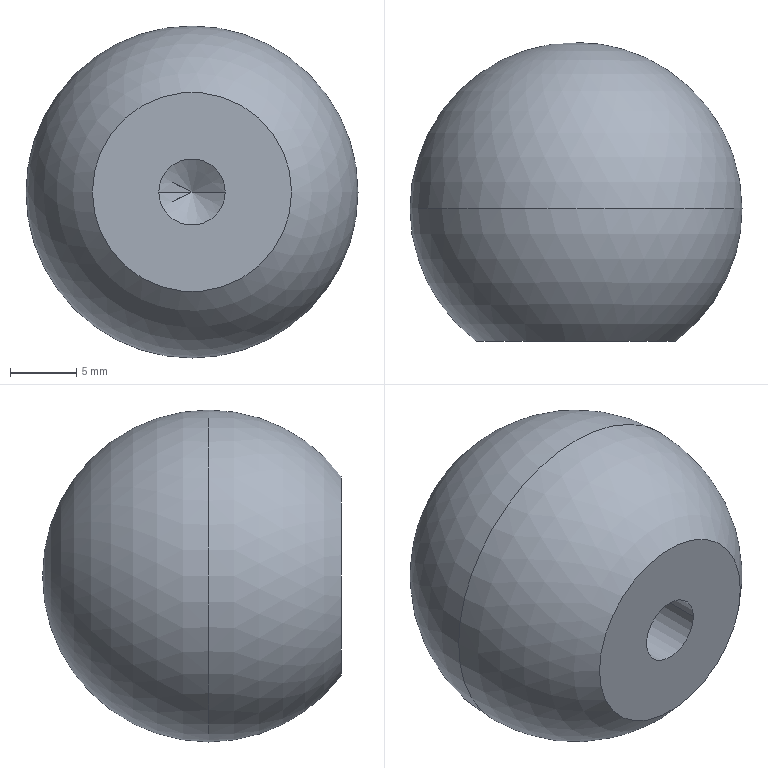Part | NX | 1 solid | 7 faces | box 25 x 22.5 x 25 mm | volume 7726 mm3 | sphere 2 | cone 2 | cylinder 2 | plane 1 | commonest cylinder face diameters 5 x2
STEP:
#1=CARTESIAN_POINT('',(-7.5,-10.,0.));
#2=VERTEX_POINT('',#1);
#3=CARTESIAN_POINT('',(7.5,-10.,0.));
#4=VERTEX_POINT('',#3);
#5=CARTESIAN_POINT('',(0.,-10.,0.));
#6=DIRECTION('',(0.,1.,0.));
#7=DIRECTION('',(-1.,0.,0.));
#8=AXIS2_PLACEMENT_3D('',#5,#6,#7);
#9=CIRCLE('',#8,7.5);
#10=EDGE_CURVE('',#2,#4,#9,.T.);
#11=ORIENTED_EDGE('',*,*,#10,.F.);
#12=CARTESIAN_POINT('',(0.,-10.,0.));
#13=DIRECTION('',(0.,1.,0.));
#14=DIRECTION('',(-1.,0.,0.));
#15=AXIS2_PLACEMENT_3D('',#12,#13,#14);
#16=CIRCLE('',#15,7.5);
#17=EDGE_CURVE('',#4,#2,#16,.T.);
#18=ORIENTED_EDGE('',*,*,#17,.F.);
#19=EDGE_LOOP('',(#11,#18));
#20=FACE_BOUND('',#19,.T.);
#21=CARTESIAN_POINT('',(-2.5,-10.,0.));
#22=VERTEX_POINT('',#21);
#23=CARTESIAN_POINT('',(2.5,-10.,0.));
#24=VERTEX_POINT('',#23);
#25=CARTESIAN_POINT('',(0.,-10.,0.));
#26=DIRECTION('',(0.,-1.,0.));
#27=DIRECTION('',(1.,0.,0.));
#28=AXIS2_PLACEMENT_3D('',#25,#26,#27);
#29=CIRCLE('',#28,2.5);
#30=EDGE_CURVE('',#22,#24,#29,.T.);
#31=ORIENTED_EDGE('',*,*,#30,.F.);
#32=CARTESIAN_POINT('',(0.,-10.,0.));
#33=DIRECTION('',(0.,-1.,0.));
#34=DIRECTION('',(1.,0.,0.));
#35=AXIS2_PLACEMENT_3D('',#32,#33,#34);
#36=CIRCLE('',#35,2.5);
#37=EDGE_CURVE('',#24,#22,#36,.T.);
#38=ORIENTED_EDGE('',*,*,#37,.F.);
#39=EDGE_LOOP('',(#31,#38));
#40=FACE_BOUND('',#39,.T.);
#41=CARTESIAN_POINT('',(0.,-10.,0.));
#42=DIRECTION('',(0.,-1.,0.));
#43=DIRECTION('',(0.,0.,-1.));
#44=AXIS2_PLACEMENT_3D('',#41,#42,#43);
#45=PLANE('',#44);
#46=ADVANCED_FACE('',(#20,#40),#45,.T.);
#47=CARTESIAN_POINT('',(12.5,0.,0.));
#48=VERTEX_POINT('',#47);
#49=CARTESIAN_POINT('',(-12.5,0.,0.));
#50=VERTEX_POINT('',#49);
#51=CARTESIAN_POINT('',(0.,0.,0.));
#52=DIRECTION('',(0.,1.,0.));
#53=DIRECTION('',(1.,0.,0.));
#54=AXIS2_PLACEMENT_3D('',#51,#52,#53);
#55=CIRCLE('',#54,12.5);
#56=EDGE_CURVE('',#48,#50,#55,.T.);
#57=ORIENTED_EDGE('',*,*,#56,.T.);
#58=CARTESIAN_POINT('',(0.,0.,0.));
#59=DIRECTION('',(0.,1.,0.));
#60=DIRECTION('',(1.,0.,0.));
#61=AXIS2_PLACEMENT_3D('',#58,#59,#60);
#62=CIRCLE('',#61,12.5);
#63=EDGE_CURVE('',#50,#48,#62,.T.);
#64=ORIENTED_EDGE('',*,*,#63,.T.);
#65=EDGE_LOOP('',(#57,#64));
#66=FACE_BOUND('',#65,.T.);
#67=CARTESIAN_POINT('',(0.,0.,0.));
#68=DIRECTION('',(0.,1.,0.));
#69=DIRECTION('',(1.,0.,0.));
#70=AXIS2_PLACEMENT_3D('',#67,#68,#69);
#71=SPHERICAL_SURFACE('',#70,12.5);
#72=ADVANCED_FACE('',(#66),#71,.T.);
#73=CARTESIAN_POINT('',(2.5,1.,0.));
#74=VERTEX_POINT('',#73);
#75=CARTESIAN_POINT('',(-2.5,1.,0.));
#76=VERTEX_POINT('',#75);
#77=CARTESIAN_POINT('',(0.,1.,0.));
#78=DIRECTION('',(0.,1.,0.));
#79=DIRECTION('',(1.,0.,0.));
#80=AXIS2_PLACEMENT_3D('',#77,#78,#79);
#81=CIRCLE('',#80,2.5);
#82=EDGE_CURVE('',#74,#76,#81,.T.);
#83=ORIENTED_EDGE('',*,*,#82,.F.);
#84=CARTESIAN_POINT('',(0.,2.502,0.));
#85=VERTEX_POINT('',#84);
#86=CARTESIAN_POINT('',(1.275,1.736,0.));
#87=DIRECTION('',(0.8572,-0.515,0.));
#88=VECTOR('',#87,1000.);
#89=LINE('',#86,#88);
#90=EDGE_CURVE('',#85,#74,#89,.T.);
#91=ORIENTED_EDGE('',*,*,#90,.F.);
#92=CARTESIAN_POINT('',(-1.275,1.736,0.));
#93=DIRECTION('',(-0.8572,-0.515,0.));
#94=VECTOR('',#93,1000.);
#95=LINE('',#92,#94);
#96=EDGE_CURVE('',#85,#76,#95,.T.);
#97=ORIENTED_EDGE('',*,*,#96,.T.);
#98=EDGE_LOOP('',(#83,#91,#97));
#99=FACE_BOUND('',#98,.T.);
#100=CARTESIAN_POINT('',(0.,1.736,0.));
#101=DIRECTION('',(0.,-1.,0.));
#102=DIRECTION('',(-1.,0.,0.));
#103=AXIS2_PLACEMENT_3D('',#100,#101,#102);
#104=CONICAL_SURFACE('',#103,1.275,1.03);
#105=ADVANCED_FACE('',(#99),#104,.F.);
#106=ORIENTED_EDGE('',*,*,#30,.T.);
#107=CARTESIAN_POINT('',(2.5,3.127,0.));
#108=DIRECTION('',(0.,-1.,0.));
#109=VECTOR('',#108,1000.);
#110=LINE('',#107,#109);
#111=EDGE_CURVE('',#24,#74,#110,.F.);
#112=ORIENTED_EDGE('',*,*,#111,.T.);
#113=ORIENTED_EDGE('',*,*,#82,.T.);
#114=CARTESIAN_POINT('',(-2.5,3.127,0.));
#115=DIRECTION('',(0.,-1.,0.));
#116=VECTOR('',#115,1000.);
#117=LINE('',#114,#116);
#118=EDGE_CURVE('',#22,#76,#117,.F.);
#119=ORIENTED_EDGE('',*,*,#118,.F.);
#120=EDGE_LOOP('',(#106,#112,#113,#119));
#121=FACE_BOUND('',#120,.T.);
#122=CARTESIAN_POINT('',(0.,3.127,0.));
#123=DIRECTION('',(0.,-1.,0.));
#124=DIRECTION('',(-1.,0.,0.));
#125=AXIS2_PLACEMENT_3D('',#122,#123,#124);
#126=CYLINDRICAL_SURFACE('',#125,2.5);
#127=ADVANCED_FACE('',(#121),#126,.F.);
#128=ORIENTED_EDGE('',*,*,#90,.T.);
#129=CARTESIAN_POINT('',(0.,1.,0.));
#130=DIRECTION('',(0.,1.,0.));
#131=DIRECTION('',(1.,0.,0.));
#132=AXIS2_PLACEMENT_3D('',#129,#130,#131);
#133=CIRCLE('',#132,2.5);
#134=EDGE_CURVE('',#76,#74,#133,.T.);
#135=ORIENTED_EDGE('',*,*,#134,.F.);
#136=ORIENTED_EDGE('',*,*,#96,.F.);
#137=EDGE_LOOP('',(#128,#135,#136));
#138=FACE_BOUND('',#137,.T.);
#139=CARTESIAN_POINT('',(0.,1.736,0.));
#140=DIRECTION('',(0.,-1.,0.));
#141=DIRECTION('',(-1.,0.,0.));
#142=AXIS2_PLACEMENT_3D('',#139,#140,#141);
#143=CONICAL_SURFACE('',#142,1.275,1.03);
#144=ADVANCED_FACE('',(#138),#143,.F.);
#145=ORIENTED_EDGE('',*,*,#118,.T.);
#146=ORIENTED_EDGE('',*,*,#134,.T.);
#147=ORIENTED_EDGE('',*,*,#111,.F.);
#148=ORIENTED_EDGE('',*,*,#37,.T.);
#149=EDGE_LOOP('',(#145,#146,#147,#148));
#150=FACE_BOUND('',#149,.T.);
#151=CARTESIAN_POINT('',(0.,3.127,0.));
#152=DIRECTION('',(0.,-1.,0.));
#153=DIRECTION('',(-1.,0.,0.));
#154=AXIS2_PLACEMENT_3D('',#151,#152,#153);
#155=CYLINDRICAL_SURFACE('',#154,2.5);
#156=ADVANCED_FACE('',(#150),#155,.F.);
#157=ORIENTED_EDGE('',*,*,#56,.F.);
#158=ORIENTED_EDGE('',*,*,#63,.F.);
#159=EDGE_LOOP('',(#157,#158));
#160=FACE_BOUND('',#159,.T.);
#161=ORIENTED_EDGE('',*,*,#10,.T.);
#162=ORIENTED_EDGE('',*,*,#17,.T.);
#163=EDGE_LOOP('',(#161,#162));
#164=FACE_BOUND('',#163,.T.);
#165=CARTESIAN_POINT('',(0.,0.,0.));
#166=DIRECTION('',(0.,1.,0.));
#167=DIRECTION('',(1.,0.,0.));
#168=AXIS2_PLACEMENT_3D('',#165,#166,#167);
#169=SPHERICAL_SURFACE('',#168,12.5);
#170=ADVANCED_FACE('',(#160,#164),#169,.T.);
#171=CLOSED_SHELL('',(#46,#72,#105,#127,#144,#156,#170));
#172=MANIFOLD_SOLID_BREP('',#171);
#173=(LENGTH_UNIT()NAMED_UNIT(*)SI_UNIT(.MILLI.,.METRE.));
#174=UNCERTAINTY_MEASURE_WITH_UNIT(LENGTH_MEASURE(0.00001),#173,'','');
#175=(NAMED_UNIT(*)PLANE_ANGLE_UNIT()SI_UNIT($,.RADIAN.));
#176=(NAMED_UNIT(*)SI_UNIT($,.STERADIAN.)SOLID_ANGLE_UNIT());
#177=(GEOMETRIC_REPRESENTATION_CONTEXT(3)GLOBAL_UNCERTAINTY_ASSIGNED_CONTEXT((#174))GLOBAL_UNIT_ASSIGNED_CONTEXT((#173,#175,#176))REPRESENTATION_CONTEXT('',''));
#178=ADVANCED_BREP_SHAPE_REPRESENTATION('',(#172),#177);